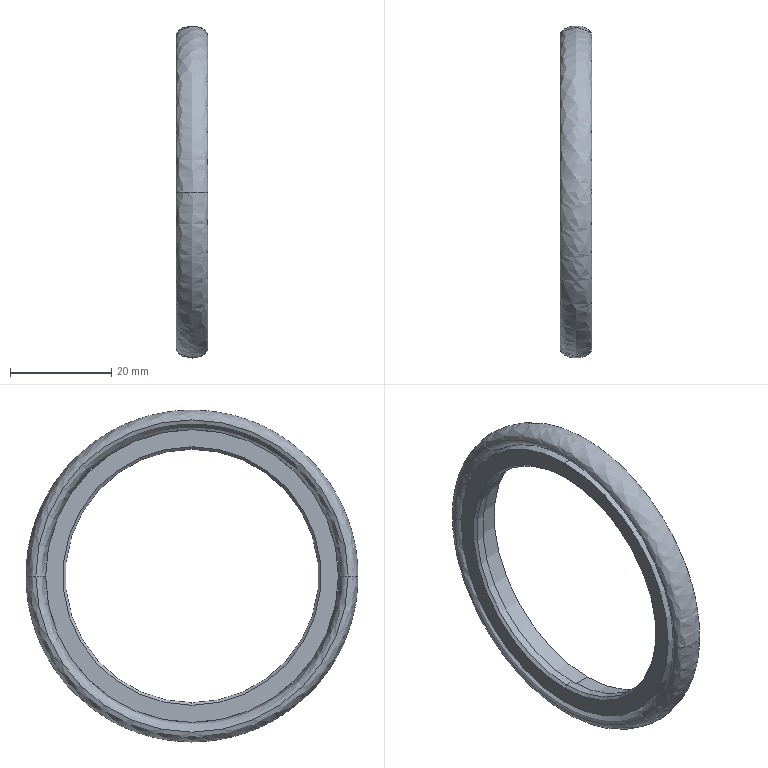Part | SolidWorks | features Revolution 3 | 2 solids | 15 faces | box 6.3 x 65.5 x 65.5 mm | volume 7151 mm3 | cylinder 6 | spline 4 | plane 3 | cone 2 | commonest cylinder face diameters 50 x2 52 x2 57.75 x2
STEP:
#1=CARTESIAN_POINT('',(6.3,0.,28.875));
#2=VERTEX_POINT('',#1);
#3=CARTESIAN_POINT('',(6.3,0.,-28.875));
#4=VERTEX_POINT('',#3);
#5=CARTESIAN_POINT('',(6.3,0.,0.));
#6=DIRECTION('',(-1.,0.,0.));
#7=DIRECTION('',(0.,0.,1.));
#8=AXIS2_PLACEMENT_3D('',#5,#6,#7);
#9=CIRCLE('',#8,28.875);
#10=EDGE_CURVE('',#2,#4,#9,.T.);
#11=ORIENTED_EDGE('',*,*,#10,.T.);
#12=CARTESIAN_POINT('',(0.,0.,-28.875));
#13=VERTEX_POINT('',#12);
#14=CARTESIAN_POINT('',(0.,0.,-28.875));
#15=DIRECTION('',(-1.,0.,0.));
#16=VECTOR('',#15,1000.);
#17=LINE('',#14,#16);
#18=EDGE_CURVE('',#4,#13,#17,.T.);
#19=ORIENTED_EDGE('',*,*,#18,.T.);
#20=CARTESIAN_POINT('',(0.,0.,28.875));
#21=VERTEX_POINT('',#20);
#22=CARTESIAN_POINT('',(0.,0.,0.));
#23=DIRECTION('',(-1.,0.,0.));
#24=DIRECTION('',(0.,0.,1.));
#25=AXIS2_PLACEMENT_3D('',#22,#23,#24);
#26=CIRCLE('',#25,28.875);
#27=EDGE_CURVE('',#21,#13,#26,.T.);
#28=ORIENTED_EDGE('',*,*,#27,.F.);
#29=CARTESIAN_POINT('',(0.,0.,28.875));
#30=DIRECTION('',(-1.,0.,0.));
#31=VECTOR('',#30,1000.);
#32=LINE('',#29,#31);
#33=EDGE_CURVE('',#2,#21,#32,.T.);
#34=ORIENTED_EDGE('',*,*,#33,.F.);
#35=EDGE_LOOP('',(#11,#19,#28,#34));
#36=FACE_OUTER_BOUND('',#35,.T.);
#37=CARTESIAN_POINT('',(0.,0.,0.));
#38=DIRECTION('',(-1.,0.,0.));
#39=DIRECTION('',(0.,0.,1.));
#40=AXIS2_PLACEMENT_3D('',#37,#38,#39);
#41=CYLINDRICAL_SURFACE('',#40,28.875);
#42=ADVANCED_FACE('',(#36),#41,.T.);
#43=CARTESIAN_POINT('',(6.3,0.,-26.));
#44=VERTEX_POINT('',#43);
#45=CARTESIAN_POINT('',(6.3,0.,26.));
#46=VERTEX_POINT('',#45);
#47=CARTESIAN_POINT('',(6.3,0.,0.));
#48=DIRECTION('',(-1.,0.,0.));
#49=DIRECTION('',(0.,0.,1.));
#50=AXIS2_PLACEMENT_3D('',#47,#48,#49);
#51=CIRCLE('',#50,26.);
#52=EDGE_CURVE('',#44,#46,#51,.T.);
#53=ORIENTED_EDGE('',*,*,#52,.F.);
#54=CARTESIAN_POINT('',(2.1,0.,-26.));
#55=VERTEX_POINT('',#54);
#56=CARTESIAN_POINT('',(0.,0.,-26.));
#57=DIRECTION('',(-1.,0.,0.));
#58=VECTOR('',#57,1000.);
#59=LINE('',#56,#58);
#60=EDGE_CURVE('',#44,#55,#59,.T.);
#61=ORIENTED_EDGE('',*,*,#60,.T.);
#62=CARTESIAN_POINT('',(2.1,0.,26.));
#63=VERTEX_POINT('',#62);
#64=CARTESIAN_POINT('',(2.1,0.,0.));
#65=DIRECTION('',(-1.,0.,0.));
#66=DIRECTION('',(0.,0.,1.));
#67=AXIS2_PLACEMENT_3D('',#64,#65,#66);
#68=CIRCLE('',#67,26.);
#69=EDGE_CURVE('',#55,#63,#68,.T.);
#70=ORIENTED_EDGE('',*,*,#69,.T.);
#71=CARTESIAN_POINT('',(0.,0.,26.));
#72=DIRECTION('',(-1.,0.,0.));
#73=VECTOR('',#72,1000.);
#74=LINE('',#71,#73);
#75=EDGE_CURVE('',#46,#63,#74,.T.);
#76=ORIENTED_EDGE('',*,*,#75,.F.);
#77=EDGE_LOOP('',(#53,#61,#70,#76));
#78=FACE_OUTER_BOUND('',#77,.T.);
#79=CARTESIAN_POINT('',(0.,0.,0.));
#80=DIRECTION('',(-1.,0.,0.));
#81=DIRECTION('',(0.,0.,1.));
#82=AXIS2_PLACEMENT_3D('',#79,#80,#81);
#83=CYLINDRICAL_SURFACE('',#82,26.);
#84=ADVANCED_FACE('',(#78),#83,.F.);
#85=CARTESIAN_POINT('',(2.1,0.,-25.));
#86=VERTEX_POINT('',#85);
#87=CARTESIAN_POINT('',(2.1,0.,25.));
#88=VERTEX_POINT('',#87);
#89=CARTESIAN_POINT('',(2.1,0.,0.));
#90=DIRECTION('',(-1.,0.,0.));
#91=DIRECTION('',(0.,0.,1.));
#92=AXIS2_PLACEMENT_3D('',#89,#90,#91);
#93=CIRCLE('',#92,25.);
#94=EDGE_CURVE('',#86,#88,#93,.T.);
#95=ORIENTED_EDGE('',*,*,#94,.F.);
#96=CARTESIAN_POINT('',(0.5,0.,-25.));
#97=VERTEX_POINT('',#96);
#98=CARTESIAN_POINT('',(0.,0.,-25.));
#99=DIRECTION('',(-1.,0.,0.));
#100=VECTOR('',#99,1000.);
#101=LINE('',#98,#100);
#102=EDGE_CURVE('',#86,#97,#101,.T.);
#103=ORIENTED_EDGE('',*,*,#102,.T.);
#104=CARTESIAN_POINT('',(0.5,0.,25.));
#105=VERTEX_POINT('',#104);
#106=CARTESIAN_POINT('',(0.5,0.,0.));
#107=DIRECTION('',(-1.,0.,0.));
#108=DIRECTION('',(0.,0.,1.));
#109=AXIS2_PLACEMENT_3D('',#106,#107,#108);
#110=CIRCLE('',#109,25.);
#111=EDGE_CURVE('',#97,#105,#110,.T.);
#112=ORIENTED_EDGE('',*,*,#111,.T.);
#113=CARTESIAN_POINT('',(0.,0.,25.));
#114=DIRECTION('',(-1.,0.,0.));
#115=VECTOR('',#114,1000.);
#116=LINE('',#113,#115);
#117=EDGE_CURVE('',#88,#105,#116,.T.);
#118=ORIENTED_EDGE('',*,*,#117,.F.);
#119=EDGE_LOOP('',(#95,#103,#112,#118));
#120=FACE_OUTER_BOUND('',#119,.T.);
#121=CARTESIAN_POINT('',(0.,0.,0.));
#122=DIRECTION('',(-1.,0.,0.));
#123=DIRECTION('',(0.,0.,1.));
#124=AXIS2_PLACEMENT_3D('',#121,#122,#123);
#125=CYLINDRICAL_SURFACE('',#124,25.);
#126=ADVANCED_FACE('',(#120),#125,.F.);
#127=ORIENTED_EDGE('',*,*,#111,.F.);
#128=CARTESIAN_POINT('',(0.,0.,-25.5));
#129=VERTEX_POINT('',#128);
#130=CARTESIAN_POINT('',(0.5,0.,-25.));
#131=DIRECTION('',(-0.7071,0.,-0.7071));
#132=VECTOR('',#131,1000.);
#133=LINE('',#130,#132);
#134=EDGE_CURVE('',#97,#129,#133,.T.);
#135=ORIENTED_EDGE('',*,*,#134,.T.);
#136=CARTESIAN_POINT('',(0.,0.,25.5));
#137=VERTEX_POINT('',#136);
#138=CARTESIAN_POINT('',(0.,0.,0.));
#139=DIRECTION('',(-1.,0.,0.));
#140=DIRECTION('',(0.,0.,1.));
#141=AXIS2_PLACEMENT_3D('',#138,#139,#140);
#142=CIRCLE('',#141,25.5);
#143=EDGE_CURVE('',#129,#137,#142,.T.);
#144=ORIENTED_EDGE('',*,*,#143,.T.);
#145=CARTESIAN_POINT('',(0.5,0.,25.));
#146=DIRECTION('',(-0.7071,0.,0.7071));
#147=VECTOR('',#146,1000.);
#148=LINE('',#145,#147);
#149=EDGE_CURVE('',#105,#137,#148,.T.);
#150=ORIENTED_EDGE('',*,*,#149,.F.);
#151=EDGE_LOOP('',(#127,#135,#144,#150));
#152=FACE_OUTER_BOUND('',#151,.T.);
#153=CARTESIAN_POINT('',(0.5,0.,0.));
#154=DIRECTION('',(-1.,0.,0.));
#155=DIRECTION('',(0.,0.,1.));
#156=AXIS2_PLACEMENT_3D('',#153,#154,#155);
#157=CONICAL_SURFACE('',#156,25.,0.7854);
#158=ADVANCED_FACE('',(#152),#157,.F.);
#159=ORIENTED_EDGE('',*,*,#134,.F.);
#160=CARTESIAN_POINT('',(0.5,0.,0.));
#161=DIRECTION('',(-1.,0.,0.));
#162=DIRECTION('',(0.,0.,1.));
#163=AXIS2_PLACEMENT_3D('',#160,#161,#162);
#164=CIRCLE('',#163,25.);
#165=EDGE_CURVE('',#105,#97,#164,.T.);
#166=ORIENTED_EDGE('',*,*,#165,.F.);
#167=ORIENTED_EDGE('',*,*,#149,.T.);
#168=CARTESIAN_POINT('',(0.,0.,0.));
#169=DIRECTION('',(-1.,0.,0.));
#170=DIRECTION('',(0.,0.,1.));
#171=AXIS2_PLACEMENT_3D('',#168,#169,#170);
#172=CIRCLE('',#171,25.5);
#173=EDGE_CURVE('',#137,#129,#172,.T.);
#174=ORIENTED_EDGE('',*,*,#173,.T.);
#175=EDGE_LOOP('',(#159,#166,#167,#174));
#176=FACE_OUTER_BOUND('',#175,.T.);
#177=CARTESIAN_POINT('',(0.5,0.,0.));
#178=DIRECTION('',(-1.,0.,0.));
#179=DIRECTION('',(0.,0.,1.));
#180=AXIS2_PLACEMENT_3D('',#177,#178,#179);
#181=CONICAL_SURFACE('',#180,25.,0.7854);
#182=ADVANCED_FACE('',(#176),#181,.F.);
#183=ORIENTED_EDGE('',*,*,#102,.F.);
#184=CARTESIAN_POINT('',(2.1,0.,0.));
#185=DIRECTION('',(-1.,0.,0.));
#186=DIRECTION('',(0.,0.,1.));
#187=AXIS2_PLACEMENT_3D('',#184,#185,#186);
#188=CIRCLE('',#187,25.);
#189=EDGE_CURVE('',#88,#86,#188,.T.);
#190=ORIENTED_EDGE('',*,*,#189,.F.);
#191=ORIENTED_EDGE('',*,*,#117,.T.);
#192=ORIENTED_EDGE('',*,*,#165,.T.);
#193=EDGE_LOOP('',(#183,#190,#191,#192));
#194=FACE_OUTER_BOUND('',#193,.T.);
#195=CARTESIAN_POINT('',(0.,0.,0.));
#196=DIRECTION('',(-1.,0.,0.));
#197=DIRECTION('',(0.,0.,1.));
#198=AXIS2_PLACEMENT_3D('',#195,#196,#197);
#199=CYLINDRICAL_SURFACE('',#198,25.);
#200=ADVANCED_FACE('',(#194),#199,.F.);
#201=ORIENTED_EDGE('',*,*,#189,.T.);
#202=ORIENTED_EDGE('',*,*,#94,.T.);
#203=EDGE_LOOP('',(#201,#202));
#204=FACE_BOUND('',#203,.T.);
#205=CARTESIAN_POINT('',(2.1,0.,0.));
#206=DIRECTION('',(-1.,0.,0.));
#207=DIRECTION('',(0.,0.,1.));
#208=AXIS2_PLACEMENT_3D('',#205,#206,#207);
#209=CIRCLE('',#208,26.);
#210=EDGE_CURVE('',#63,#55,#209,.T.);
#211=ORIENTED_EDGE('',*,*,#210,.F.);
#212=ORIENTED_EDGE('',*,*,#69,.F.);
#213=EDGE_LOOP('',(#211,#212));
#214=FACE_OUTER_BOUND('',#213,.T.);
#215=CARTESIAN_POINT('',(2.1,0.,0.));
#216=DIRECTION('',(1.,0.,0.));
#217=DIRECTION('',(0.,0.,-1.));
#218=AXIS2_PLACEMENT_3D('',#215,#216,#217);
#219=PLANE('',#218);
#220=ADVANCED_FACE('',(#204,#214),#219,.T.);
#221=ORIENTED_EDGE('',*,*,#60,.F.);
#222=CARTESIAN_POINT('',(6.3,0.,0.));
#223=DIRECTION('',(-1.,0.,0.));
#224=DIRECTION('',(0.,0.,1.));
#225=AXIS2_PLACEMENT_3D('',#222,#223,#224);
#226=CIRCLE('',#225,26.);
#227=EDGE_CURVE('',#46,#44,#226,.T.);
#228=ORIENTED_EDGE('',*,*,#227,.F.);
#229=ORIENTED_EDGE('',*,*,#75,.T.);
#230=ORIENTED_EDGE('',*,*,#210,.T.);
#231=EDGE_LOOP('',(#221,#228,#229,#230));
#232=FACE_OUTER_BOUND('',#231,.T.);
#233=CARTESIAN_POINT('',(0.,0.,0.));
#234=DIRECTION('',(-1.,0.,0.));
#235=DIRECTION('',(0.,0.,1.));
#236=AXIS2_PLACEMENT_3D('',#233,#234,#235);
#237=CYLINDRICAL_SURFACE('',#236,26.);
#238=ADVANCED_FACE('',(#232),#237,.F.);
#239=ORIENTED_EDGE('',*,*,#10,.F.);
#240=CARTESIAN_POINT('',(6.3,0.,0.));
#241=DIRECTION('',(-1.,0.,0.));
#242=DIRECTION('',(0.,0.,1.));
#243=AXIS2_PLACEMENT_3D('',#240,#241,#242);
#244=CIRCLE('',#243,28.875);
#245=EDGE_CURVE('',#4,#2,#244,.T.);
#246=ORIENTED_EDGE('',*,*,#245,.F.);
#247=EDGE_LOOP('',(#239,#246));
#248=FACE_OUTER_BOUND('',#247,.T.);
#249=ORIENTED_EDGE('',*,*,#227,.T.);
#250=ORIENTED_EDGE('',*,*,#52,.T.);
#251=EDGE_LOOP('',(#249,#250));
#252=FACE_BOUND('',#251,.T.);
#253=CARTESIAN_POINT('',(6.3,0.,0.));
#254=DIRECTION('',(-1.,0.,0.));
#255=DIRECTION('',(0.,0.,1.));
#256=AXIS2_PLACEMENT_3D('',#253,#254,#255);
#257=PLANE('',#256);
#258=ADVANCED_FACE('',(#248,#252),#257,.F.);
#259=ORIENTED_EDGE('',*,*,#18,.F.);
#260=ORIENTED_EDGE('',*,*,#245,.T.);
#261=ORIENTED_EDGE('',*,*,#33,.T.);
#262=CARTESIAN_POINT('',(0.,0.,0.));
#263=DIRECTION('',(-1.,0.,0.));
#264=DIRECTION('',(0.,0.,1.));
#265=AXIS2_PLACEMENT_3D('',#262,#263,#264);
#266=CIRCLE('',#265,28.875);
#267=EDGE_CURVE('',#13,#21,#266,.T.);
#268=ORIENTED_EDGE('',*,*,#267,.F.);
#269=EDGE_LOOP('',(#259,#260,#261,#268));
#270=FACE_OUTER_BOUND('',#269,.T.);
#271=CARTESIAN_POINT('',(0.,0.,0.));
#272=DIRECTION('',(-1.,0.,0.));
#273=DIRECTION('',(0.,0.,1.));
#274=AXIS2_PLACEMENT_3D('',#271,#272,#273);
#275=CYLINDRICAL_SURFACE('',#274,28.875);
#276=ADVANCED_FACE('',(#270),#275,.T.);
#277=ORIENTED_EDGE('',*,*,#27,.T.);
#278=ORIENTED_EDGE('',*,*,#267,.T.);
#279=EDGE_LOOP('',(#277,#278));
#280=FACE_OUTER_BOUND('',#279,.T.);
#281=ORIENTED_EDGE('',*,*,#173,.F.);
#282=ORIENTED_EDGE('',*,*,#143,.F.);
#283=EDGE_LOOP('',(#281,#282));
#284=FACE_BOUND('',#283,.T.);
#285=CARTESIAN_POINT('',(0.,0.,0.));
#286=DIRECTION('',(-1.,0.,0.));
#287=DIRECTION('',(0.,0.,1.));
#288=AXIS2_PLACEMENT_3D('',#285,#286,#287);
#289=PLANE('',#288);
#290=ADVANCED_FACE('',(#280,#284),#289,.T.);
#291=CLOSED_SHELL('',(#42,#84,#126,#158,#182,#200,#220,#238,#258,#276,#290));
#292=MANIFOLD_SOLID_BREP('',#291);
#293=CARTESIAN_POINT('',(0.,30.812,0.));
#294=VERTEX_POINT('',#293);
#295=CARTESIAN_POINT('',(0.,-30.812,0.));
#296=VERTEX_POINT('',#295);
#297=CARTESIAN_POINT('',(0.,0.,0.));
#298=DIRECTION('',(-1.,0.,0.));
#299=DIRECTION('',(0.,1.,0.));
#300=AXIS2_PLACEMENT_3D('',#297,#298,#299);
#301=CIRCLE('',#300,30.812);
#302=EDGE_CURVE('',#294,#296,#301,.T.);
#303=ORIENTED_EDGE('',*,*,#302,.T.);
#304=CARTESIAN_POINT('',(6.3,-30.812,0.));
#305=VERTEX_POINT('',#304);
#306=CARTESIAN_POINT('',(0.,-30.812,0.));
#307=CARTESIAN_POINT('',(0.,-26.937,0.));
#308=CARTESIAN_POINT('',(6.3,-26.937,0.));
#309=CARTESIAN_POINT('',(6.3,-30.812,0.));
#310=(BOUNDED_CURVE()B_SPLINE_CURVE(3,(#306,#307,#308,#309),.UNSPECIFIED.,.F.,.F.)B_SPLINE_CURVE_WITH_KNOTS((4,4),(0.,3.142),.UNSPECIFIED.)CURVE()GEOMETRIC_REPRESENTATION_ITEM()RATIONAL_B_SPLINE_CURVE((1.,0.3333,0.3333,1.))REPRESENTATION_ITEM(''));
#311=EDGE_CURVE('',#296,#305,#310,.T.);
#312=ORIENTED_EDGE('',*,*,#311,.T.);
#313=CARTESIAN_POINT('',(6.3,30.812,0.));
#314=VERTEX_POINT('',#313);
#315=CARTESIAN_POINT('',(6.3,0.,0.));
#316=DIRECTION('',(-1.,0.,0.));
#317=DIRECTION('',(0.,1.,0.));
#318=AXIS2_PLACEMENT_3D('',#315,#316,#317);
#319=CIRCLE('',#318,30.812);
#320=EDGE_CURVE('',#314,#305,#319,.T.);
#321=ORIENTED_EDGE('',*,*,#320,.F.);
#322=CARTESIAN_POINT('',(0.,30.812,0.));
#323=CARTESIAN_POINT('',(0.,26.937,0.));
#324=CARTESIAN_POINT('',(6.3,26.937,0.));
#325=CARTESIAN_POINT('',(6.3,30.812,0.));
#326=(BOUNDED_CURVE()B_SPLINE_CURVE(3,(#322,#323,#324,#325),.UNSPECIFIED.,.F.,.F.)B_SPLINE_CURVE_WITH_KNOTS((4,4),(0.,3.142),.UNSPECIFIED.)CURVE()GEOMETRIC_REPRESENTATION_ITEM()RATIONAL_B_SPLINE_CURVE((1.,0.3333,0.3333,1.))REPRESENTATION_ITEM(''));
#327=EDGE_CURVE('',#294,#314,#326,.T.);
#328=ORIENTED_EDGE('',*,*,#327,.F.);
#329=EDGE_LOOP('',(#303,#312,#321,#328));
#330=FACE_OUTER_BOUND('',#329,.T.);
#331=CARTESIAN_POINT('',(0.,30.812,0.));
#332=CARTESIAN_POINT('',(0.,30.813,-61.625));
#333=CARTESIAN_POINT('',(0.,-30.812,-61.625));
#334=CARTESIAN_POINT('',(0.,-30.812,0.));
#335=CARTESIAN_POINT('',(0.,26.937,0.));
#336=CARTESIAN_POINT('',(0.,26.937,-53.875));
#337=CARTESIAN_POINT('',(0.,-26.937,-53.875));
#338=CARTESIAN_POINT('',(0.,-26.937,0.));
#339=CARTESIAN_POINT('',(6.3,26.937,0.));
#340=CARTESIAN_POINT('',(6.3,26.937,-53.875));
#341=CARTESIAN_POINT('',(6.3,-26.937,-53.875));
#342=CARTESIAN_POINT('',(6.3,-26.937,0.));
#343=CARTESIAN_POINT('',(6.3,30.812,0.));
#344=CARTESIAN_POINT('',(6.3,30.813,-61.625));
#345=CARTESIAN_POINT('',(6.3,-30.812,-61.625));
#346=CARTESIAN_POINT('',(6.3,-30.812,0.));
#347=(BOUNDED_SURFACE()B_SPLINE_SURFACE(3,3,((#331,#332,#333,#334),(#335,#336,#337,#338),(#339,#340,#341,#342),(#343,#344,#345,#346)),.UNSPECIFIED.,.F.,.F.,.F.)B_SPLINE_SURFACE_WITH_KNOTS((4,4),(4,4),(0.,1.),(0.,1.),.UNSPECIFIED.)GEOMETRIC_REPRESENTATION_ITEM()RATIONAL_B_SPLINE_SURFACE(((1.,0.3333,0.3333,1.),(0.3333,0.1111,0.1111,0.3333),(0.3333,0.1111,0.1111,0.3333),(1.,0.3333,0.3333,1.)))REPRESENTATION_ITEM('')SURFACE());
#348=ADVANCED_FACE('',(#330),#347,.F.);
#349=ORIENTED_EDGE('',*,*,#320,.T.);
#350=CARTESIAN_POINT('',(6.3,-30.812,0.));
#351=CARTESIAN_POINT('',(6.3,-34.688,0.));
#352=CARTESIAN_POINT('',(0.,-34.688,0.));
#353=CARTESIAN_POINT('',(0.,-30.812,0.));
#354=(BOUNDED_CURVE()B_SPLINE_CURVE(3,(#350,#351,#352,#353),.UNSPECIFIED.,.F.,.T.)B_SPLINE_CURVE_WITH_KNOTS((4,4),(3.142,6.283),.UNSPECIFIED.)CURVE()GEOMETRIC_REPRESENTATION_ITEM()RATIONAL_B_SPLINE_CURVE((1.,0.3333,0.3333,1.))REPRESENTATION_ITEM(''));
#355=EDGE_CURVE('',#305,#296,#354,.T.);
#356=ORIENTED_EDGE('',*,*,#355,.T.);
#357=ORIENTED_EDGE('',*,*,#302,.F.);
#358=CARTESIAN_POINT('',(6.3,30.812,0.));
#359=CARTESIAN_POINT('',(6.3,34.688,0.));
#360=CARTESIAN_POINT('',(0.,34.688,0.));
#361=CARTESIAN_POINT('',(0.,30.812,0.));
#362=(BOUNDED_CURVE()B_SPLINE_CURVE(3,(#358,#359,#360,#361),.UNSPECIFIED.,.F.,.F.)B_SPLINE_CURVE_WITH_KNOTS((4,4),(3.142,6.283),.UNSPECIFIED.)CURVE()GEOMETRIC_REPRESENTATION_ITEM()RATIONAL_B_SPLINE_CURVE((1.,0.3333,0.3333,1.))REPRESENTATION_ITEM(''));
#363=EDGE_CURVE('',#314,#294,#362,.T.);
#364=ORIENTED_EDGE('',*,*,#363,.F.);
#365=EDGE_LOOP('',(#349,#356,#357,#364));
#366=FACE_OUTER_BOUND('',#365,.T.);
#367=CARTESIAN_POINT('',(6.3,30.812,0.));
#368=CARTESIAN_POINT('',(6.3,30.813,-61.625));
#369=CARTESIAN_POINT('',(6.3,-30.812,-61.625));
#370=CARTESIAN_POINT('',(6.3,-30.812,0.));
#371=CARTESIAN_POINT('',(6.3,34.688,0.));
#372=CARTESIAN_POINT('',(6.3,34.688,-69.375));
#373=CARTESIAN_POINT('',(6.3,-34.688,-69.375));
#374=CARTESIAN_POINT('',(6.3,-34.688,0.));
#375=CARTESIAN_POINT('',(0.,34.688,0.));
#376=CARTESIAN_POINT('',(0.,34.688,-69.375));
#377=CARTESIAN_POINT('',(0.,-34.688,-69.375));
#378=CARTESIAN_POINT('',(0.,-34.688,0.));
#379=CARTESIAN_POINT('',(0.,30.812,0.));
#380=CARTESIAN_POINT('',(0.,30.813,-61.625));
#381=CARTESIAN_POINT('',(0.,-30.812,-61.625));
#382=CARTESIAN_POINT('',(0.,-30.812,0.));
#383=(BOUNDED_SURFACE()B_SPLINE_SURFACE(3,3,((#367,#368,#369,#370),(#371,#372,#373,#374),(#375,#376,#377,#378),(#379,#380,#381,#382)),.UNSPECIFIED.,.F.,.F.,.T.)B_SPLINE_SURFACE_WITH_KNOTS((4,4),(4,4),(0.,1.),(0.,1.),.UNSPECIFIED.)GEOMETRIC_REPRESENTATION_ITEM()RATIONAL_B_SPLINE_SURFACE(((1.,0.3333,0.3333,1.),(0.3333,0.1111,0.1111,0.3333),(0.3333,0.1111,0.1111,0.3333),(1.,0.3333,0.3333,1.)))REPRESENTATION_ITEM('')SURFACE());
#384=ADVANCED_FACE('',(#366),#383,.F.);
#385=ORIENTED_EDGE('',*,*,#355,.F.);
#386=CARTESIAN_POINT('',(6.3,0.,0.));
#387=DIRECTION('',(-1.,0.,0.));
#388=DIRECTION('',(0.,1.,0.));
#389=AXIS2_PLACEMENT_3D('',#386,#387,#388);
#390=CIRCLE('',#389,30.812);
#391=EDGE_CURVE('',#305,#314,#390,.T.);
#392=ORIENTED_EDGE('',*,*,#391,.T.);
#393=ORIENTED_EDGE('',*,*,#363,.T.);
#394=CARTESIAN_POINT('',(0.,0.,0.));
#395=DIRECTION('',(-1.,0.,0.));
#396=DIRECTION('',(0.,1.,0.));
#397=AXIS2_PLACEMENT_3D('',#394,#395,#396);
#398=CIRCLE('',#397,30.812);
#399=EDGE_CURVE('',#296,#294,#398,.T.);
#400=ORIENTED_EDGE('',*,*,#399,.F.);
#401=EDGE_LOOP('',(#385,#392,#393,#400));
#402=FACE_OUTER_BOUND('',#401,.T.);
#403=CARTESIAN_POINT('',(6.3,-30.812,0.));
#404=CARTESIAN_POINT('',(6.3,-30.813,61.625));
#405=CARTESIAN_POINT('',(6.3,30.812,61.625));
#406=CARTESIAN_POINT('',(6.3,30.812,0.));
#407=CARTESIAN_POINT('',(6.3,-34.688,0.));
#408=CARTESIAN_POINT('',(6.3,-34.688,69.375));
#409=CARTESIAN_POINT('',(6.3,34.688,69.375));
#410=CARTESIAN_POINT('',(6.3,34.688,0.));
#411=CARTESIAN_POINT('',(0.,-34.688,0.));
#412=CARTESIAN_POINT('',(0.,-34.688,69.375));
#413=CARTESIAN_POINT('',(0.,34.688,69.375));
#414=CARTESIAN_POINT('',(0.,34.688,0.));
#415=CARTESIAN_POINT('',(0.,-30.812,0.));
#416=CARTESIAN_POINT('',(0.,-30.813,61.625));
#417=CARTESIAN_POINT('',(0.,30.812,61.625));
#418=CARTESIAN_POINT('',(0.,30.812,0.));
#419=(BOUNDED_SURFACE()B_SPLINE_SURFACE(3,3,((#403,#404,#405,#406),(#407,#408,#409,#410),(#411,#412,#413,#414),(#415,#416,#417,#418)),.UNSPECIFIED.,.F.,.F.,.T.)B_SPLINE_SURFACE_WITH_KNOTS((4,4),(4,4),(0.,1.),(0.,1.),.UNSPECIFIED.)GEOMETRIC_REPRESENTATION_ITEM()RATIONAL_B_SPLINE_SURFACE(((1.,0.3333,0.3333,1.),(0.3333,0.1111,0.1111,0.3333),(0.3333,0.1111,0.1111,0.3333),(1.,0.3333,0.3333,1.)))REPRESENTATION_ITEM('')SURFACE());
#420=ADVANCED_FACE('',(#402),#419,.F.);
#421=ORIENTED_EDGE('',*,*,#311,.F.);
#422=ORIENTED_EDGE('',*,*,#399,.T.);
#423=ORIENTED_EDGE('',*,*,#327,.T.);
#424=ORIENTED_EDGE('',*,*,#391,.F.);
#425=EDGE_LOOP('',(#421,#422,#423,#424));
#426=FACE_OUTER_BOUND('',#425,.T.);
#427=CARTESIAN_POINT('',(0.,-30.812,0.));
#428=CARTESIAN_POINT('',(0.,-30.813,61.625));
#429=CARTESIAN_POINT('',(0.,30.812,61.625));
#430=CARTESIAN_POINT('',(0.,30.812,0.));
#431=CARTESIAN_POINT('',(0.,-26.937,0.));
#432=CARTESIAN_POINT('',(0.,-26.937,53.875));
#433=CARTESIAN_POINT('',(0.,26.937,53.875));
#434=CARTESIAN_POINT('',(0.,26.937,0.));
#435=CARTESIAN_POINT('',(6.3,-26.937,0.));
#436=CARTESIAN_POINT('',(6.3,-26.937,53.875));
#437=CARTESIAN_POINT('',(6.3,26.937,53.875));
#438=CARTESIAN_POINT('',(6.3,26.937,0.));
#439=CARTESIAN_POINT('',(6.3,-30.812,0.));
#440=CARTESIAN_POINT('',(6.3,-30.813,61.625));
#441=CARTESIAN_POINT('',(6.3,30.812,61.625));
#442=CARTESIAN_POINT('',(6.3,30.812,0.));
#443=(BOUNDED_SURFACE()B_SPLINE_SURFACE(3,3,((#427,#428,#429,#430),(#431,#432,#433,#434),(#435,#436,#437,#438),(#439,#440,#441,#442)),.UNSPECIFIED.,.F.,.F.,.T.)B_SPLINE_SURFACE_WITH_KNOTS((4,4),(4,4),(0.,1.),(0.,1.),.UNSPECIFIED.)GEOMETRIC_REPRESENTATION_ITEM()RATIONAL_B_SPLINE_SURFACE(((1.,0.3333,0.3333,1.),(0.3333,0.1111,0.1111,0.3333),(0.3333,0.1111,0.1111,0.3333),(1.,0.3333,0.3333,1.)))REPRESENTATION_ITEM('')SURFACE());
#444=ADVANCED_FACE('',(#426),#443,.F.);
#445=CLOSED_SHELL('',(#348,#384,#420,#444));
#446=MANIFOLD_SOLID_BREP('',#445);
#447=CARTESIAN_POINT('',(0.,0.,0.));
#448=DIRECTION('',(0.,0.,1.));
#449=DIRECTION('',(1.,0.,0.));
#450=AXIS2_PLACEMENT_3D('',#447,#448,#449);
#451=(LENGTH_UNIT()NAMED_UNIT(*)SI_UNIT(.MILLI.,.METRE.));
#452=UNCERTAINTY_MEASURE_WITH_UNIT(LENGTH_MEASURE(0.00001),#451,'','');
#453=(NAMED_UNIT(*)PLANE_ANGLE_UNIT()SI_UNIT($,.RADIAN.));
#454=(NAMED_UNIT(*)SI_UNIT($,.STERADIAN.)SOLID_ANGLE_UNIT());
#455=(GEOMETRIC_REPRESENTATION_CONTEXT(3)GLOBAL_UNCERTAINTY_ASSIGNED_CONTEXT((#452))GLOBAL_UNIT_ASSIGNED_CONTEXT((#451,#453,#454))REPRESENTATION_CONTEXT('',''));
#456=ADVANCED_BREP_SHAPE_REPRESENTATION('',(#292,#446,#450),#455);